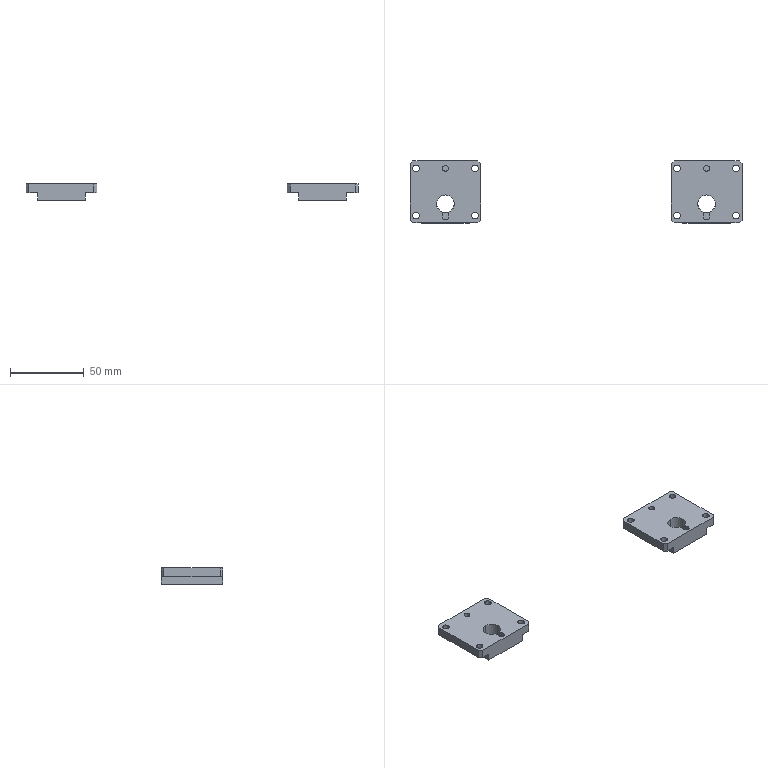NC program | NX | posted with a generic post | part box 225 x 42 x 11 mm
Whole program:
N10 G17 G21 G94 G90
(FLOOR_WALL , TOOL : D63)
N12 T01 M6
N14 G54
N16 G17 G0 G90 X-60.5 Y0. S6500 M3
N18 G43 Z30. H1
N20 Z3.
N22 G94 G1 Z0. F1500.
N24 X-57.5
N26 X57.5
N28 X60.5
N30 Z3.
N32 G0 Z30.
N34 M5
(DRILLING , TOOL : D6A45)
N36 T07 M6
N38 G54
N40 G17 G0 G90 X20. Y-16. S5000 M3
N42 G43 Z30. H7
N44 G94 G81 G98 Z-1. F250. R3.
N46 Y16.
N48 X0.
N50 X-20.
N52 Y-16.
N54 G80
N56 G0 X-20. Y-16. Z30.
N58 M5
(DRILLING_COPY , TOOL : 4.5ZT)
N60 T14 M6
N62 G54
N64 G17 G0 G90 X20. Y-16. S2000 M3
N66 G43 Z30. H14
N68 G94 G83 G98 Z-8.852 F250. Q2. R3.
N70 Y16.
N72 X-20.
N74 Y-16.
N76 G80
N78 G0 X-20. Y-16. Z30.
N80 M5
(ZLEVEL_PROFILE , TOOL : D10)
N82 T10 M6
N84 G54
N86 G17 G0 G90 X1.406 Y-26.1 S9500 M3
N88 G43 Z30. H10
N90 Z1.5
N92 G94 G1 X-22. Z0.273 F1000.
N94 X-22.554 Z0.244
N96 X-23.963 Y-25.74 Z0.168
N98 X-25.215 Y-24.998 Z0.092
N100 X-27.998 Y-22.215 Z-0.114
N102 X-28.74 Y-20.963 Z-0.191
N104 X-29.1 Y-19.554 Z-0.267
N106 Y-19. Z-0.296
N108 Y19. F3000.
N110 G2 X-27.606 Y22.606 R5.1
N112 G1 X-25.606 Y24.606
N114 G2 X-22. Y26.1 R5.1
N116 G1 X22.
N118 G2 X25.606 Y24.606 R5.1
N120 G1 X27.606 Y22.606
N122 G2 X29.1 Y19. R5.1
N124 G1 Y-19.
N126 G2 X27.606 Y-22.606 R5.1
N128 G1 X25.606 Y-24.606
N130 G2 X22. Y-26.1 R5.1
N132 G1 X-22.
N134 G2 X-25.606 Y-24.606 R5.1
N136 G1 X-27.606 Y-22.606
N138 G2 X-29.1 Y-19. R5.1
N140 G1 Y-2.045 Z-0.592
N142 Y19.
N144 G2 X-27.606 Y22.606 R5.1
N146 G1 X-25.606 Y24.606
N148 G2 X-22. Y26.1 R5.1
N150 G1 X22.
N152 G2 X25.606 Y24.606 R5.1
N154 G1 X27.606 Y22.606
N156 G2 X29.1 Y19. R5.1
N158 G1 Y-19.
N160 G2 X27.606 Y-22.606 R5.1
N162 G1 X25.606 Y-24.606
N164 G2 X22. Y-26.1 R5.1
N166 G1 X-22.
N168 G2 X-25.606 Y-24.606 R5.1
N170 G1 X-27.606 Y-22.606
N172 G2 X-29.1 Y-19. R5.1
N174 G1 Y-2.045 Z-0.888
N176 Y19.
N178 G2 X-27.606 Y22.606 R5.1
N180 G1 X-25.606 Y24.606
N182 G2 X-22. Y26.1 R5.1
N184 G1 X22.
N186 G2 X25.606 Y24.606 R5.1
N188 G1 X27.606 Y22.606
N190 G2 X29.1 Y19. R5.1
N192 G1 Y-19.
N194 G2 X27.606 Y-22.606 R5.1
N196 G1 X25.606 Y-24.606
N198 G2 X22. Y-26.1 R5.1
N200 G1 X-22.
N202 G2 X-25.606 Y-24.606 R5.1
N204 G1 X-27.606 Y-22.606
N206 G2 X-29.1 Y-19. R5.1
N208 G1 Y-2.045 Z-1.184
N210 Y19.
N212 G2 X-27.606 Y22.606 R5.1
N214 G1 X-25.606 Y24.606
N216 G2 X-22. Y26.1 R5.1
N218 G1 X22.
N220 G2 X25.606 Y24.606 R5.1
N222 G1 X27.606 Y22.606
N224 G2 X29.1 Y19. R5.1
N226 G1 Y-19.
N228 G2 X27.606 Y-22.606 R5.1
N230 G1 X25.606 Y-24.606
N232 G2 X22. Y-26.1 R5.1
N234 G1 X-22.
N236 G2 X-25.606 Y-24.606 R5.1
N238 G1 X-27.606 Y-22.606
N240 G2 X-29.1 Y-19. R5.1
N242 G1 Y-2.045 Z-1.48
N244 Y19.
N246 G2 X-27.606 Y22.606 R5.1
N248 G1 X-25.606 Y24.606
N250 G2 X-22. Y26.1 R5.1
N252 G1 X22.
N254 G2 X25.606 Y24.606 R5.1
N256 G1 X27.606 Y22.606
N258 G2 X29.1 Y19. R5.1
N260 G1 Y-19.
N262 G2 X27.606 Y-22.606 R5.1
N264 G1 X25.606 Y-24.606
N266 G2 X22. Y-26.1 R5.1
N268 G1 X-22.
N270 G2 X-25.606 Y-24.606 R5.1
N272 G1 X-27.606 Y-22.606
N274 G2 X-29.1 Y-19. R5.1
N276 G1 Y-2.045 Z-1.776
N278 Y19.
N280 G2 X-27.606 Y22.606 R5.1
N282 G1 X-25.606 Y24.606
N284 G2 X-22. Y26.1 R5.1
N286 G1 X22.
N288 G2 X25.606 Y24.606 R5.1
N290 G1 X27.606 Y22.606
N292 G2 X29.1 Y19. R5.1
N294 G1 Y-19.
N296 G2 X27.606 Y-22.606 R5.1
N298 G1 X25.606 Y-24.606
N300 G2 X22. Y-26.1 R5.1
N302 G1 X-22.
N304 G2 X-25.606 Y-24.606 R5.1
N306 G1 X-27.606 Y-22.606
N308 G2 X-29.1 Y-19. R5.1
N310 G1 Y-2.045 Z-2.072
N312 Y19.
N314 G2 X-27.606 Y22.606 R5.1
N316 G1 X-25.606 Y24.606
N318 G2 X-22. Y26.1 R5.1
N320 G1 X22.
N322 G2 X25.606 Y24.606 R5.1
N324 G1 X27.606 Y22.606
N326 G2 X29.1 Y19. R5.1
N328 G1 Y-19.
N330 G2 X27.606 Y-22.606 R5.1
N332 G1 X25.606 Y-24.606
N334 G2 X22. Y-26.1 R5.1
N336 G1 X-22.
N338 G2 X-25.606 Y-24.606 R5.1
N340 G1 X-27.606 Y-22.606
N342 G2 X-29.1 Y-19. R5.1
N344 G1 Y-2.045 Z-2.368
N346 Y19.
N348 G2 X-27.606 Y22.606 R5.1
N350 G1 X-25.606 Y24.606
N352 G2 X-22. Y26.1 R5.1
N354 G1 X22.
N356 G2 X25.606 Y24.606 R5.1
N358 G1 X27.606 Y22.606
N360 G2 X29.1 Y19. R5.1
N362 G1 Y-19.
N364 G2 X27.606 Y-22.606 R5.1
N366 G1 X25.606 Y-24.606
N368 G2 X22. Y-26.1 R5.1
N370 G1 X-22.
N372 G2 X-25.606 Y-24.606 R5.1
N374 G1 X-27.606 Y-22.606
N376 G2 X-29.1 Y-19. R5.1
N378 G1 Y-2.045 Z-2.664
N380 Y19.
N382 G2 X-27.606 Y22.606 R5.1
N384 G1 X-25.606 Y24.606
N386 G2 X-22. Y26.1 R5.1
N388 G1 X22.
N390 G2 X25.606 Y24.606 R5.1
N392 G1 X27.606 Y22.606
N394 G2 X29.1 Y19. R5.1
N396 G1 Y-19.
N398 G2 X27.606 Y-22.606 R5.1
N400 G1 X25.606 Y-24.606
N402 G2 X22. Y-26.1 R5.1
N404 G1 X-22.
N406 G2 X-25.606 Y-24.606 R5.1
N408 G1 X-27.606 Y-22.606
N410 G2 X-29.1 Y-19. R5.1
N412 G1 Y-2.045 Z-2.959
N414 Y19.
N416 G2 X-27.606 Y22.606 R5.1
N418 G1 X-25.606 Y24.606
N420 G2 X-22. Y26.1 R5.1
N422 G1 X22.
N424 G2 X25.606 Y24.606 R5.1
N426 G1 X27.606 Y22.606
N428 G2 X29.1 Y19. R5.1
N430 G1 Y-19.
N432 G2 X27.606 Y-22.606 R5.1
N434 G1 X25.606 Y-24.606
N436 G2 X22. Y-26.1 R5.1
N438 G1 X-22.
N440 G2 X-25.606 Y-24.606 R5.1
N442 G1 X-27.606 Y-22.606
N444 G2 X-29.1 Y-19. R5.1
N446 G1 Y-2.045 Z-3.255
N448 Y19.
N450 G2 X-27.606 Y22.606 R5.1
N452 G1 X-25.606 Y24.606
N454 G2 X-22. Y26.1 R5.1
N456 G1 X22.
N458 G2 X25.606 Y24.606 R5.1
N460 G1 X27.606 Y22.606
N462 G2 X29.1 Y19. R5.1
N464 G1 Y-19.
N466 G2 X27.606 Y-22.606 R5.1
N468 G1 X25.606 Y-24.606
N470 G2 X22. Y-26.1 R5.1
N472 G1 X-22.
N474 G2 X-25.606 Y-24.606 R5.1
N476 G1 X-27.606 Y-22.606
N478 G2 X-29.1 Y-19. R5.1
N480 G1 Y-2.045 Z-3.551
N482 Y19.
N484 G2 X-27.606 Y22.606 R5.1
N486 G1 X-25.606 Y24.606
N488 G2 X-22. Y26.1 R5.1
N490 G1 X22.
N492 G2 X25.606 Y24.606 R5.1
N494 G1 X27.606 Y22.606
N496 G2 X29.1 Y19. R5.1
N498 G1 Y-19.
N500 G2 X27.606 Y-22.606 R5.1
N502 G1 X25.606 Y-24.606
N504 G2 X22. Y-26.1 R5.1
N506 G1 X-22.
N508 G2 X-25.606 Y-24.606 R5.1
N510 G1 X-27.606 Y-22.606
N512 G2 X-29.1 Y-19. R5.1
N514 G1 Y-2.045 Z-3.847
N516 Y19.
N518 G2 X-27.606 Y22.606 R5.1
N520 G1 X-25.606 Y24.606
N522 G2 X-22. Y26.1 R5.1
N524 G1 X22.
N526 G2 X25.606 Y24.606 R5.1
N528 G1 X27.606 Y22.606
N530 G2 X29.1 Y19. R5.1
N532 G1 Y-19.
N534 G2 X27.606 Y-22.606 R5.1
N536 G1 X25.606 Y-24.606
N538 G2 X22. Y-26.1 R5.1
N540 G1 X-22.
N542 G2 X-25.606 Y-24.606 R5.1
N544 G1 X-27.606 Y-22.606
N546 G2 X-29.1 Y-19. R5.1
N548 G1 Y-2.045 Z-4.143
N550 Y19.
N552 G2 X-27.606 Y22.606 R5.1
N554 G1 X-25.606 Y24.606
N556 G2 X-22. Y26.1 R5.1
N558 G1 X22.
N560 G2 X25.606 Y24.606 R5.1
N562 G1 X27.606 Y22.606
N564 G2 X29.1 Y19. R5.1
N566 G1 Y-19.
N568 G2 X27.606 Y-22.606 R5.1
N570 G1 X25.606 Y-24.606
N572 G2 X22. Y-26.1 R5.1
N574 G1 X-22.
N576 G2 X-25.606 Y-24.606 R5.1
N578 G1 X-27.606 Y-22.606
N580 G2 X-29.1 Y-19. R5.1
N582 G1 Y-2.045 Z-4.439
N584 Y19.
N586 G2 X-27.606 Y22.606 R5.1
N588 G1 X-25.606 Y24.606
N590 G2 X-22. Y26.1 R5.1
N592 G1 X22.
N594 G2 X25.606 Y24.606 R5.1
N596 G1 X27.606 Y22.606
N598 G2 X29.1 Y19. R5.1
N600 G1 Y-19.
N602 G2 X27.606 Y-22.606 R5.1
N604 G1 X25.606 Y-24.606
N606 G2 X22. Y-26.1 R5.1
N608 G1 X-22.
N610 G2 X-25.606 Y-24.606 R5.1
N612 G1 X-27.606 Y-22.606
N614 G2 X-29.1 Y-19. R5.1
N616 G1 Y-2.045 Z-4.735
N618 Y19.
N620 G2 X-27.606 Y22.606 R5.1
N622 G1 X-25.606 Y24.606
N624 G2 X-22. Y26.1 R5.1
N626 G1 X22.
N628 G2 X25.606 Y24.606 R5.1
N630 G1 X27.606 Y22.606
N632 G2 X29.1 Y19. R5.1
N634 G1 Y-19.
N636 G2 X27.606 Y-22.606 R5.1
N638 G1 X25.606 Y-24.606
N640 G2 X22. Y-26.1 R5.1
N642 G1 X-22.
N644 G2 X-25.606 Y-24.606 R5.1
N646 G1 X-27.606 Y-22.606
N648 G2 X-29.1 Y-19. R5.1
N650 G1 Y-2.045 Z-5.031
N652 Y19.
N654 G2 X-27.606 Y22.606 R5.1
N656 G1 X-25.606 Y24.606
N658 G2 X-22. Y26.1 R5.1
N660 G1 X22.
N662 G2 X25.606 Y24.606 R5.1
N664 G1 X27.606 Y22.606
N666 G2 X29.1 Y19. R5.1
N668 G1 Y-19.
N670 G2 X27.606 Y-22.606 R5.1
N672 G1 X25.606 Y-24.606
N674 G2 X22. Y-26.1 R5.1
N676 G1 X-22.
N678 G2 X-25.606 Y-24.606 R5.1
N680 G1 X-27.606 Y-22.606
N682 G2 X-29.1 Y-19. R5.1
N684 G1 Y-2.045 Z-5.327
N686 Y19.
N688 G2 X-27.606 Y22.606 R5.1
N690 G1 X-25.606 Y24.606
N692 G2 X-22. Y26.1 R5.1
N694 G1 X22.
N696 G2 X25.606 Y24.606 R5.1
N698 G1 X27.606 Y22.606
N700 G2 X29.1 Y19. R5.1
N702 G1 Y-19.
N704 G2 X27.606 Y-22.606 R5.1
N706 G1 X25.606 Y-24.606
N708 G2 X22. Y-26.1 R5.1
N710 G1 X-22.
N712 G2 X-25.606 Y-24.606 R5.1
N714 G1 X-27.606 Y-22.606
N716 G2 X-29.1 Y-19. R5.1
N718 G1 Y-2.045 Z-5.623
N720 Y19.
N722 G2 X-27.606 Y22.606 R5.1
N724 G1 X-25.606 Y24.606
N726 G2 X-22. Y26.1 R5.1
N728 G1 X22.
N730 G2 X25.606 Y24.606 R5.1
N732 G1 X27.606 Y22.606
N734 G2 X29.1 Y19. R5.1
N736 G1 Y-19.
N738 G2 X27.606 Y-22.606 R5.1
N740 G1 X25.606 Y-24.606
N742 G2 X22. Y-26.1 R5.1
N744 G1 X-22.
N746 G2 X-25.606 Y-24.606 R5.1
N748 G1 X-27.606 Y-22.606
N750 G2 X-29.1 Y-19. R5.1
N752 G1 Y-2.045 Z-5.919
N754 Y19.
N756 G2 X-27.606 Y22.606 R5.1
N758 G1 X-25.606 Y24.606
N760 G2 X-22. Y26.1 R5.1
N762 G1 X22.
N764 G2 X25.606 Y24.606 R5.1
N766 G1 X27.606 Y22.606
N768 G2 X29.1 Y19. R5.1
N770 G1 Y-19.
N772 G2 X27.606 Y-22.606 R5.1
N774 G1 X25.606 Y-24.606
N776 G2 X22. Y-26.1 R5.1
N778 G1 X-22.
N780 G2 X-25.606 Y-24.606 R5.1
N782 G1 X-27.606 Y-22.606
N784 G2 X-29.1 Y-19. R5.1
N786 G1 Y-2.045 Z-6.215
N788 Y19.
N790 G2 X-27.606 Y22.606 R5.1
N792 G1 X-25.606 Y24.606
N794 G2 X-22. Y26.1 R5.1
N796 G1 X22.
N798 G2 X25.606 Y24.606 R5.1
N800 G1 X27.606 Y22.606
N802 G2 X29.1 Y19. R5.1
N804 G1 Y-19.
N806 G2 X27.606 Y-22.606 R5.1
N808 G1 X25.606 Y-24.606
N810 G2 X22. Y-26.1 R5.1
N812 G1 X-22.
N814 G2 X-25.606 Y-24.606 R5.1
N816 G1 X-27.606 Y-22.606
N818 G2 X-29.1 Y-19. R5.1
N820 G1 Y-2.045 Z-6.511
N822 Y19.
N824 G2 X-27.606 Y22.606 R5.1
N826 G1 X-25.606 Y24.606
N828 G2 X-22. Y26.1 R5.1
N830 G1 X22.
N832 G2 X25.606 Y24.606 R5.1
N834 G1 X27.606 Y22.606
N836 G2 X29.1 Y19. R5.1
N838 G1 Y-19.
N840 G2 X27.606 Y-22.606 R5.1
N842 G1 X25.606 Y-24.606
N844 G2 X22. Y-26.1 R5.1
N846 G1 X-22.
N848 G2 X-25.606 Y-24.606 R5.1
N850 G1 X-27.606 Y-22.606
N852 G2 X-29.1 Y-19. R5.1
N854 G1 Y-2.045 Z-6.807
N856 Y19.
N858 G2 X-27.606 Y22.606 R5.1
N860 G1 X-25.606 Y24.606
N862 G2 X-22. Y26.1 R5.1
N864 G1 X22.
N866 G2 X25.606 Y24.606 R5.1
N868 G1 X27.606 Y22.606
N870 G2 X29.1 Y19. R5.1
N872 G1 Y-19.
N874 G2 X27.606 Y-22.606 R5.1
N876 G1 X25.606 Y-24.606
N878 G2 X22. Y-26.1 R5.1
N880 G1 X-22.
N882 G2 X-25.606 Y-24.606 R5.1
N884 G1 X-27.606 Y-22.606
N886 G2 X-29.1 Y-19. R5.1
N888 G1 Y-2.045 Z-7.103
N890 Y19.
N892 G2 X-27.606 Y22.606 R5.1
N894 G1 X-25.606 Y24.606
N896 G2 X-22. Y26.1 R5.1
N898 G1 X22.
N900 G2 X25.606 Y24.606 R5.1
N902 G1 X27.606 Y22.606
N904 G2 X29.1 Y19. R5.1
N906 G1 Y-19.
N908 G2 X27.606 Y-22.606 R5.1
N910 G1 X25.606 Y-24.606
N912 G2 X22. Y-26.1 R5.1
N914 G1 X-22.
N916 G2 X-25.606 Y-24.606 R5.1
N918 G1 X-27.606 Y-22.606
N920 G2 X-29.1 Y-19. R5.1
N922 G1 Y-2.045 Z-7.399
N924 Y19.
N926 G2 X-27.606 Y22.606 R5.1
N928 G1 X-25.606 Y24.606
N930 G2 X-22. Y26.1 R5.1
N932 G1 X22.
N934 G2 X25.606 Y24.606 R5.1
N936 G1 X27.606 Y22.606
N938 G2 X29.1 Y19. R5.1
N940 G1 Y-19.
N942 G2 X27.606 Y-22.606 R5.1
N944 G1 X25.606 Y-24.606
N946 G2 X22. Y-26.1 R5.1
N948 G1 X-22.
N950 G2 X-25.606 Y-24.606 R5.1
N952 G1 X-27.606 Y-22.606
N954 G2 X-29.1 Y-19. R5.1
N956 G1 Y-2.045 Z-7.695
N958 Y19.
N960 G2 X-27.606 Y22.606 R5.1
N962 G1 X-25.606 Y24.606
N964 G2 X-22. Y26.1 R5.1
N966 G1 X22.
N968 G2 X25.606 Y24.606 R5.1
N970 G1 X27.606 Y22.606
N972 G2 X29.1 Y19. R5.1
N974 G1 Y-19.
N976 G2 X27.606 Y-22.606 R5.1
N978 G1 X25.606 Y-24.606
N980 G2 X22. Y-26.1 R5.1
N982 G1 X-22.
N984 G2 X-25.606 Y-24.606 R5.1
N986 G1 X-27.606 Y-22.606
N988 G2 X-29.1 Y-19. R5.1
N990 G1 Y-2.045 Z-7.991
N992 Y19.
N994 G2 X-27.606 Y22.606 R5.1
N996 G1 X-25.606 Y24.606
N998 G2 X-22. Y26.1 R5.1
N1000 G1 X22.
N1002 G2 X25.606 Y24.606 R5.1
N1004 G1 X27.606 Y22.606
N1006 G2 X29.1 Y19. R5.1
N1008 G1 Y-19.
N1010 G2 X27.606 Y-22.606 R5.1
N1012 G1 X25.606 Y-24.606
N1014 G2 X22. Y-26.1 R5.1
N1016 G1 X-22.
N1018 G2 X-25.606 Y-24.606 R5.1
N1020 G1 X-27.606 Y-22.606
N1022 G2 X-29.1 Y-19. R5.1
N1024 G1 Y-2.045 Z-8.286
N1026 Y19.
N1028 G2 X-27.606 Y22.606 R5.1
N1030 G1 X-25.606 Y24.606
N1032 G2 X-22. Y26.1 R5.1
N1034 G1 X22.
N1036 G2 X25.606 Y24.606 R5.1
N1038 G1 X27.606 Y22.606
N1040 G2 X29.1 Y19. R5.1
N1042 G1 Y-19.
N1044 G2 X27.606 Y-22.606 R5.1
N1046 G1 X25.606 Y-24.606
N1048 G2 X22. Y-26.1 R5.1
N1050 G1 X-22.
N1052 G2 X-25.606 Y-24.606 R5.1
N1054 G1 X-27.606 Y-22.606
N1056 G2 X-29.1 Y-19. R5.1
N1058 G1 Y-2.045 Z-8.582
N1060 Y19.
N1062 G2 X-27.606 Y22.606 R5.1
N1064 G1 X-25.606 Y24.606
N1066 G2 X-22. Y26.1 R5.1
N1068 G1 X22.
N1070 G2 X25.606 Y24.606 R5.1
N1072 G1 X27.606 Y22.606
N1074 G2 X29.1 Y19. R5.1
N1076 G1 Y-19.
N1078 G2 X27.606 Y-22.606 R5.1
N1080 G1 X25.606 Y-24.606
N1082 G2 X22. Y-26.1 R5.1
N1084 G1 X-22.
N1086 G2 X-25.606 Y-24.606 R5.1
N1088 G1 X-27.606 Y-22.606
N1090 G2 X-29.1 Y-19. R5.1
N1092 G1 Y-2.045 Z-8.878
N1094 Y19.
N1096 G2 X-27.606 Y22.606 R5.1
N1098 G1 X-25.606 Y24.606
N1100 G2 X-22. Y26.1 R5.1
N1102 G1 X22.
N1104 G2 X25.606 Y24.606 R5.1
N1106 G1 X27.606 Y22.606
N1108 G2 X29.1 Y19. R5.1
N1110 G1 Y-19.
N1112 G2 X27.606 Y-22.606 R5.1
N1114 G1 X25.606 Y-24.606
N1116 G2 X22. Y-26.1 R5.1
N1118 G1 X-22.
N1120 G2 X-25.606 Y-24.606 R5.1
N1122 G1 X-27.606 Y-22.606
N1124 G2 X-29.1 Y-19. R5.1
N1126 G1 Y-2.045 Z-9.174
N1128 Y19.
N1130 G2 X-27.606 Y22.606 R5.1
N1132 G1 X-25.606 Y24.606
N1134 G2 X-22. Y26.1 R5.1
N1136 G1 X22.
N1138 G2 X25.606 Y24.606 R5.1
N1140 G1 X27.606 Y22.606
N1142 G2 X29.1 Y19. R5.1
N1144 G1 Y-19.
N1146 G2 X27.606 Y-22.606 R5.1
N1148 G1 X25.606 Y-24.606
N1150 G2 X22. Y-26.1 R5.1
N1152 G1 X-22.
N1154 G2 X-25.606 Y-24.606 R5.1
N1156 G1 X-27.606 Y-22.606
N1158 G2 X-29.1 Y-19. R5.1
N1160 G1 Y-2.045 Z-9.47
N1162 Y19.
N1164 G2 X-27.606 Y22.606 R5.1
N1166 G1 X-25.606 Y24.606
N1168 G2 X-22. Y26.1 R5.1
N1170 G1 X22.
N1172 G2 X25.606 Y24.606 R5.1
N1174 G1 X27.606 Y22.606
N1176 G2 X29.1 Y19. R5.1
N1178 G1 Y-19.
N1180 G2 X27.606 Y-22.606 R5.1
N1182 G1 X25.606 Y-24.606
N1184 G2 X22. Y-26.1 R5.1
N1186 G1 X-22.
N1188 G2 X-25.606 Y-24.606 R5.1
N1190 G1 X-27.606 Y-22.606
N1192 G2 X-29.1 Y-19. R5.1
N1194 G1 Y-2.045 Z-9.766
N1196 Y19.
N1198 G2 X-27.606 Y22.606 R5.1
N1200 G1 X-25.606 Y24.606
N1202 G2 X-22. Y26.1 R5.1
N1204 G1 X22.
N1206 G2 X25.606 Y24.606 R5.1
N1208 G1 X27.606 Y22.606
N1210 G2 X29.1 Y19. R5.1
N1212 G1 Y-19.
N1214 G2 X27.606 Y-22.606 R5.1
N1216 G1 X25.606 Y-24.606
N1218 G2 X22. Y-26.1 R5.1
N1220 G1 X-22.
N1222 G2 X-25.606 Y-24.606 R5.1
N1224 G1 X-27.606 Y-22.606
N1226 G2 X-29.1 Y-19. R5.1
N1228 G1 Y-2.045 Z-10.062
N1230 Y19.
N1232 G2 X-27.606 Y22.606 R5.1
N1234 G1 X-25.606 Y24.606
N1236 G2 X-22. Y26.1 R5.1
N1238 G1 X22.
N1240 G2 X25.606 Y24.606 R5.1
N1242 G1 X27.606 Y22.606
N1244 G2 X29.1 Y19. R5.1
N1246 G1 Y-19.
N1248 G2 X27.606 Y-22.606 R5.1
N1250 G1 X25.606 Y-24.606
N1252 G2 X22. Y-26.1 R5.1
N1254 G1 X-22.
N1256 G2 X-25.606 Y-24.606 R5.1
N1258 G1 X-27.606 Y-22.606
N1260 G2 X-29.1 Y-19. R5.1
N1262 G1 Y-2.045 Z-10.358
N1264 Y19.
N1266 G2 X-27.606 Y22.606 R5.1
N1268 G1 X-25.606 Y24.606
N1270 G2 X-22. Y26.1 R5.1
N1272 G1 X22.
N1274 G2 X25.606 Y24.606 R5.1
N1276 G1 X27.606 Y22.606
N1278 G2 X29.1 Y19. R5.1
N1280 G1 Y-19.
N1282 G2 X27.606 Y-22.606 R5.1
N1284 G1 X25.606 Y-24.606
N1286 G2 X22. Y-26.1 R5.1
N1288 G1 X-22.
N1290 G2 X-25.606 Y-24.606 R5.1
N1292 G1 X-27.606 Y-22.606
N1294 G2 X-29.1 Y-19. R5.1
N1296 G1 Y-2.045 Z-10.654
N1298 Y19.
N1300 G2 X-27.606 Y22.606 R5.1
N1302 G1 X-25.606 Y24.606
N1304 G2 X-22. Y26.1 R5.1
N1306 G1 X22.
N1308 G2 X25.606 Y24.606 R5.1
N1310 G1 X27.606 Y22.606
N1312 G2 X29.1 Y19. R5.1
N1314 G1 Y-19.
N1316 G2 X27.606 Y-22.606 R5.1
N1318 G1 X25.606 Y-24.606
N1320 G2 X22. Y-26.1 R5.1
N1322 G1 X-22.
N1324 G2 X-25.606 Y-24.606 R5.1
N1326 G1 X-27.606 Y-22.606
N1328 G2 X-29.1 Y-19. R5.1
N1330 G1 Y-2.045 Z-10.95
N1332 Y19.
N1334 G2 X-27.606 Y22.606 R5.1
N1336 G1 X-25.606 Y24.606
N1338 G2 X-22. Y26.1 R5.1
N1340 G1 X22.
N1342 G2 X25.606 Y24.606 R5.1
N1344 G1 X27.606 Y22.606
N1346 G2 X29.1 Y19. R5.1
N1348 G1 Y-19.
N1350 G2 X27.606 Y-22.606 R5.1
N1352 G1 X25.606 Y-24.606
N1354 G2 X22. Y-26.1 R5.1
N1356 G1 X-22.
N1358 G2 X-25.606 Y-24.606 R5.1
N1360 G1 X-27.606 Y-22.606
N1362 G2 X-29.1 Y-19. R5.1
N1364 G1 Y-2.045
N1366 Z-9.45
N1368 G0 Z30.
(HOLE_MILLING , TOOL : D10)
N1370 X0. Y-8.
N1372 Z0.5
N1374 G3 X0.45 Y-8.45 R0.45 F2000.
N1376 X0.9 Y-8. R0.45
N1378 X0.9 Y-8. Z0.2 I-0.9 J0.
N1380 X0.9 Y-8. Z-0.1 I-0.9 J0.
N1382 X0.9 Y-8. Z-0.4 I-0.9 J0.
N1384 X0.9 Y-8. Z-0.7 I-0.9 J0.
N1386 X0.9 Y-8. Z-1. I-0.9 J0.
N1388 X0.9 Y-8. Z-1.3 I-0.9 J0.
N1390 X0.9 Y-8. Z-1.6 I-0.9 J0.
N1392 X0.9 Y-8. Z-1.9 I-0.9 J0.
N1394 X0.9 Y-8. Z-2.2 I-0.9 J0.
N1396 X0.9 Y-8. Z-2.5 I-0.9 J0.
N1398 X0.9 Y-8. Z-2.8 I-0.9 J0.
N1400 X0.9 Y-8. Z-3.1 I-0.9 J0.
N1402 X0.9 Y-8. Z-3.4 I-0.9 J0.
N1404 X0.9 Y-8. Z-3.7 I-0.9 J0.
N1406 X0.9 Y-8. Z-4. I-0.9 J0.
N1408 X0.9 Y-8. Z-4.3 I-0.9 J0.
N1410 X0.9 Y-8. Z-4.6 I-0.9 J0.
N1412 X0.9 Y-8. Z-4.9 I-0.9 J0.
N1414 X0.9 Y-8. Z-5.2 I-0.9 J0.
N1416 X0.9 Y-8. Z-5.5 I-0.9 J0.
N1418 X0.9 Y-8. Z-5.8 I-0.9 J0.
N1420 X0.9 Y-8. Z-6.1 I-0.9 J0.
N1422 X0.9 Y-8. Z-6.4 I-0.9 J0.
N1424 X0.9 Y-8. Z-6.7 I-0.9 J0.
N1426 X0.9 Y-8. Z-7. I-0.9 J0.
N1428 X0.9 Y-8. Z-7.3 I-0.9 J0.
N1430 X0.9 Y-8. Z-7.6 I-0.9 J0.
N1432 X0.9 Y-8. Z-7.9 I-0.9 J0.
N1434 X0.9 Y-8. Z-8.2 I-0.9 J0.
N1436 X0.9 Y-8. Z-8.5 I-0.9 J0.
N1438 X0.9 Y-8. Z-8.8 I-0.9 J0.
N1440 X0.9 Y-8. Z-9.1 I-0.9 J0.
N1442 X0.9 Y-8. Z-9.4 I-0.9 J0.
N1444 X0.9 Y-8. Z-9.7 I-0.9 J0.
N1446 X0.9 Y-8. Z-10. I-0.9 J0.
N1448 X0.9 Y-8. Z-10.3 I-0.9 J0.
N1450 X0.9 Y-8. Z-10.6 I-0.9 J0.
N1452 X0.9 Y-8. Z-10.9 I-0.9 J0.
N1454 X-0.45 Y-7.221 Z-11. R0.9
N1456 X-0.779 Y-8.45 R0.9
N1458 X-0.45 Y-7.221 R-0.9
N1460 X-0.615 Y-7.835 R0.45
N1462 X0. Y-8. R0.45
N1464 G0 Z30.
N1466 M5
(HOLE_MILLING_COPY , TOOL : D10JING)
N1468 T11 M6
N1470 G54
N1472 G17 G0 G90 X0. Y-8. S9500 M3
N1474 G43 Z30. H11
N1476 Z0.5
N1478 G94 G3 X0.5 Y-8.5 R0.5 F1200.
N1480 X1. Y-8. R0.5
N1482 X1. Y-8. Z-4.5 I-1. J0.
N1484 X1. Y-8. Z-9.5 I-1. J0.
N1486 X-0.309 Y-7.049 Z-11. R1.
N1488 X-0.951 Y-8.309 R1.
N1490 X-0.309 Y-7.049 R-1.
N1492 X-0.63 Y-7.679 R0.5
N1494 X0. Y-8. R0.5
N1496 G0 Z30.
N1498 M5
(HOLE_MILLING_1 , TOOL : D3)
N1500 T03 M6
N1502 G54
N1504 G17 G0 G90 X0. Y16. S9500 M3
N1506 G43 Z30. H3
N1508 Z0.5
N1510 G94 G3 X0.2 Y15.8 R0.2 F1250.
N1512 X0.4 Y16. R0.2
N1514 X0.4 Y16. Z0.35 I-0.4 J0.
N1516 X0.4 Y16. Z0.2 I-0.4 J0.
N1518 X0.4 Y16. Z0.05 I-0.4 J0.
N1520 X0.4 Y16. Z-0.1 I-0.4 J0.
N1522 X0.4 Y16. Z-0.25 I-0.4 J0.
N1524 X0.4 Y16. Z-0.4 I-0.4 J0.
N1526 X0.4 Y16. Z-0.55 I-0.4 J0.
N1528 X0.4 Y16. Z-0.7 I-0.4 J0.
N1530 X0.4 Y16. Z-0.85 I-0.4 J0.
N1532 X0.4 Y16. Z-1. I-0.4 J0.
N1534 X0.4 Y16. Z-1.15 I-0.4 J0.
N1536 X0.4 Y16. Z-1.3 I-0.4 J0.
N1538 X0.4 Y16. Z-1.45 I-0.4 J0.
N1540 X0.4 Y16. Z-1.6 I-0.4 J0.
N1542 X0.4 Y16. Z-1.75 I-0.4 J0.
N1544 X0.4 Y16. Z-1.9 I-0.4 J0.
N1546 X0.4 Y16. Z-2.05 I-0.4 J0.
N1548 X0.4 Y16. Z-2.2 I-0.4 J0.
N1550 X0.4 Y16. Z-2.35 I-0.4 J0.
N1552 X0.4 Y16. Z-2.5 I-0.4 J0.
N1554 X0.4 Y16. Z-2.65 I-0.4 J0.
N1556 X0.4 Y16. Z-2.8 I-0.4 J0.
N1558 X0.4 Y16. Z-2.95 I-0.4 J0.
N1560 X0.4 Y16. Z-3.1 I-0.4 J0.
N1562 X0.4 Y16. Z-3.25 I-0.4 J0.
N1564 X0.4 Y16. Z-3.4 I-0.4 J0.
N1566 X0.4 Y16. Z-3.55 I-0.4 J0.
N1568 X0.4 Y16. Z-3.7 I-0.4 J0.
N1570 X0.4 Y16. Z-3.85 I-0.4 J0.
N1572 X0.4 Y16. Z-4. I-0.4 J0.
N1574 X0.4 Y16. Z-4.15 I-0.4 J0.
N1576 X0.4 Y16. Z-4.3 I-0.4 J0.
N1578 X0.4 Y16. Z-4.45 I-0.4 J0.
N1580 X0.4 Y16. Z-4.6 I-0.4 J0.
N1582 X0.4 Y16. Z-4.75 I-0.4 J0.
N1584 X0.4 Y16. Z-4.9 I-0.4 J0.
N1586 X0.4 Y16. Z-5.05 I-0.4 J0.
N1588 X0.4 Y16. Z-5.2 I-0.4 J0.
N1590 X0.4 Y16. Z-5.35 I-0.4 J0.
N1592 X0.4 Y16. Z-5.5 I-0.4 J0.
N1594 X0.4 Y16. Z-5.65 I-0.4 J0.
N1596 X0.4 Y16. Z-5.8 I-0.4 J0.
N1598 X0.4 Y16. Z-5.95 I-0.4 J0.
N1600 X-0.2 Y16.346 Z-6. R0.4
N1602 X-0.346 Y15.8 R0.4
N1604 X-0.2 Y16.346 R-0.4
N1606 X-0.273 Y16.073 R0.2
N1608 X0. Y16. R0.2
N1610 G0 Z30.
(ZLEVEL_PROFILE_1 , TOOL : D3)
N1612 Y-11.097
N1614 Z-0.15
N1616 G1 X-0.256 Y-11.895 F1500.
N1618 G3 X-0.403 Y-12.157 R0.3
N1620 G1 X-0.4 Y-12.41
N1622 Y-13.667
N1624 Y-17.
N1626 G3 X0. Y-17.4 R0.4
N1628 X0.4 Y-17. R0.4
N1630 G1 Y-13.657
N1632 X0.419 Y-13.408
N1634 X0.4 Y-13.389
N1636 X0.403 Y-12.157
N1638 G3 X0.254 Y-11.897 R0.3
N1640 G1 X0. Y-11.097
N1642 G0 Z-0.3
N1644 G1 X-0.255 Y-11.895
N1646 G3 X-0.403 Y-12.157 R0.3
N1648 G1 X-0.4 Y-12.41
N1650 Y-13.667
N1652 Y-17.
N1654 G3 X0. Y-17.4 R0.4
N1656 X0.4 Y-17. R0.4
N1658 G1 Y-13.657
N1660 X0.419 Y-13.408
N1662 X0.4 Y-13.389
N1664 X0.403 Y-12.157
N1666 G3 X0.254 Y-11.897 R0.3
N1668 G1 X0. Y-11.097
N1670 G0 Y-11.096 Z-0.45
N1672 G1 X-0.255 Y-11.896
N1674 G3 X-0.402 Y-12.157 R0.3
N1676 G1 X-0.4 Y-12.41
N1678 Y-13.667
N1680 Y-17.
N1682 G3 X0. Y-17.4 R0.4
N1684 X0.4 Y-17. R0.4
N1686 G1 Y-13.657
N1688 X0.419 Y-13.408
N1690 X0.4 Y-13.389
N1692 X0.403 Y-12.157
N1694 G3 X0.253 Y-11.897 R0.3
N1696 G1 X0. Y-11.096
N1698 G0 Z-0.6
N1700 G1 X-0.255 Y-11.896
N1702 G3 X-0.402 Y-12.157 R0.3
N1704 G1 X-0.4 Y-12.41
N1706 Y-13.667
N1708 Y-17.
N1710 G3 X0. Y-17.4 R0.4
N1712 X0.4 Y-17. R0.4
N1714 G1 Y-13.657
N1716 X0.419 Y-13.408
N1718 X0.4 Y-13.389
N1720 X0.403 Y-12.157
N1722 G3 X0.253 Y-11.897 R0.3
N1724 G1 X0. Y-11.096
N1726 G0 Z-0.75
N1728 G1 X-0.255 Y-11.896
N1730 G3 X-0.402 Y-12.157 R0.3
N1732 G1 X-0.4 Y-12.41
N1734 Y-13.667
N1736 Y-17.
N1738 G3 X0. Y-17.4 R0.4
N1740 X0.4 Y-17. R0.4
N1742 G1 Y-13.657
N1744 X0.419 Y-13.408
N1746 X0.4 Y-13.389
N1748 X0.403 Y-12.157
N1750 G3 X0.253 Y-11.897 R0.3
N1752 G1 X0. Y-11.096
N1754 G0 Z-0.9
N1756 G1 X-0.255 Y-11.896
N1758 G3 X-0.402 Y-12.157 R0.3
N1760 G1 X-0.4 Y-12.41
N1762 Y-13.667
N1764 Y-17.
N1766 G3 X0. Y-17.4 R0.4
N1768 X0.4 Y-17. R0.4
N1770 G1 Y-13.657
N1772 X0.419 Y-13.408
N1774 X0.4 Y-13.389
N1776 X0.403 Y-12.157
N1778 G3 X0.253 Y-11.897 R0.3
N1780 G1 X0. Y-11.096
N1782 G0 Z-1.05
N1784 G1 X-0.255 Y-11.896
N1786 G3 X-0.402 Y-12.157 R0.3
N1788 G1 X-0.399 Y-12.41
N1790 X-0.4 Y-13.667
N1792 Y-17.
N1794 G3 X0. Y-17.4 R0.4
N1796 X0.4 Y-17. R0.4
N1798 G1 X0.399 Y-13.657
N1800 X0.419 Y-13.408
N1802 X0.399 Y-13.389
N1804 X0.403 Y-12.157
N1806 G3 X0.253 Y-11.897 R0.3
N1808 G1 X0. Y-11.096
N1810 G0 Z-1.2
N1812 G1 X-0.255 Y-11.896
N1814 G3 X-0.402 Y-12.157 R0.3
N1816 G1 X-0.399 Y-12.41
N1818 X-0.4 Y-13.667
N1820 Y-17.
N1822 G3 X0. Y-17.4 R0.4
N1824 X0.4 Y-17. R0.4
N1826 G1 X0.399 Y-13.657
N1828 X0.419 Y-13.408
N1830 X0.399 Y-13.389
N1832 X0.403 Y-12.157
N1834 G3 X0.253 Y-11.897 R0.3
N1836 G1 X0. Y-11.096
N1838 G0 Z-1.35
N1840 G1 X-0.255 Y-11.896
N1842 G3 X-0.402 Y-12.157 R0.3
N1844 G1 X-0.399 Y-12.41
N1846 X-0.4 Y-13.667
N1848 Y-17.
N1850 G3 X0. Y-17.4 R0.4
N1852 X0.4 Y-17. R0.4
N1854 G1 X0.399 Y-13.657
N1856 X0.419 Y-13.408
N1858 X0.399 Y-13.389
N1860 X0.403 Y-12.157
N1862 G3 X0.253 Y-11.897 R0.3
N1864 G1 X0. Y-11.096
N1866 G0 Z-1.5
N1868 G1 X-0.255 Y-11.896
N1870 G3 X-0.402 Y-12.157 R0.3
N1872 G1 X-0.399 Y-12.41
N1874 X-0.4 Y-13.667
N1876 Y-17.
N1878 G3 X0. Y-17.4 R0.4
N1880 X0.4 Y-17. R0.4
N1882 G1 X0.399 Y-13.657
N1884 X0.419 Y-13.408
N1886 X0.399 Y-13.389
N1888 X0.403 Y-12.157
N1890 G3 X0.253 Y-11.897 R0.3
N1892 G1 X0. Y-11.096
N1894 G0 Z-1.65
N1896 G1 X-0.255 Y-11.896
N1898 G3 X-0.402 Y-12.157 R0.3
N1900 G1 X-0.399 Y-12.41
N1902 X-0.4 Y-13.667
N1904 Y-17.
N1906 G3 X0. Y-17.4 R0.4
N1908 X0.4 Y-17. R0.4
N1910 G1 X0.399 Y-13.657
N1912 X0.419 Y-13.408
N1914 X0.399 Y-13.389
N1916 X0.403 Y-12.157
N1918 G3 X0.253 Y-11.897 R0.3
N1920 G1 X0. Y-11.096
N1922 G0 Z-1.8
N1924 G1 X-0.255 Y-11.896
N1926 G3 X-0.402 Y-12.157 R0.3
N1928 G1 X-0.399 Y-12.41
N1930 X-0.4 Y-13.667
N1932 Y-17.
N1934 G3 X0. Y-17.4 R0.4
N1936 X0.4 Y-17. R0.4
N1938 G1 X0.399 Y-13.657
N1940 X0.419 Y-13.408
N1942 X0.399 Y-13.389
N1944 X0.403 Y-12.157
N1946 G3 X0.253 Y-11.897 R0.3
N1948 G1 X0. Y-11.096
N1950 G0 Y-11.095 Z-1.95
N1952 G1 X-0.255 Y-11.896
N1954 G3 X-0.402 Y-12.157 R0.3
N1956 G1 X-0.399 Y-12.41
N1958 X-0.4 Y-13.667
N1960 Y-17.
N1962 G3 X0. Y-17.4 R0.4
N1964 X0.4 Y-17. R0.4
N1966 G1 X0.399 Y-13.657
N1968 X0.419 Y-13.408
N1970 X0.399 Y-13.389
N1972 X0.403 Y-12.157
N1974 G3 X0.253 Y-11.897 R0.3
N1976 G1 X0. Y-11.095
N1978 G0 Z-2.1
N1980 G1 X-0.255 Y-11.896
N1982 G3 X-0.402 Y-12.157 R0.3
N1984 G1 X-0.399 Y-12.41
N1986 X-0.4 Y-13.667
N1988 Y-17.
N1990 G3 X0. Y-17.4 R0.4
N1992 X0.4 Y-17. R0.4
N1994 G1 X0.399 Y-13.657
N1996 X0.419 Y-13.408
N1998 X0.399 Y-13.389
N2000 X0.403 Y-12.157
N2002 G3 X0.253 Y-11.897 R0.3
N2004 G1 X0. Y-11.095
N2006 G0 Z-2.25
N2008 G1 X-0.255 Y-11.896
N2010 G3 X-0.402 Y-12.157 R0.3
N2012 G1 X-0.399 Y-12.41
N2014 X-0.4 Y-13.667
N2016 Y-17.
N2018 G3 X0. Y-17.4 R0.4
N2020 X0.4 Y-17. R0.4
N2022 G1 X0.399 Y-13.657
N2024 X0.419 Y-13.408
N2026 X0.399 Y-13.389
N2028 X0.402 Y-12.157
N2030 G3 X0.253 Y-11.897 R0.3
N2032 G1 X0. Y-11.095
N2034 G0 Z-2.4
N2036 G1 X-0.255 Y-11.896
N2038 G3 X-0.402 Y-12.157 R0.3
N2040 G1 X-0.399 Y-12.41
N2042 X-0.4 Y-13.667
N2044 Y-17.
N2046 G3 X0. Y-17.4 R0.4
N2048 X0.4 Y-17. R0.4
N2050 G1 X0.399 Y-13.657
N2052 X0.419 Y-13.408
N2054 X0.399 Y-13.389
N2056 X0.402 Y-12.157
N2058 G3 X0.253 Y-11.897 R0.3
N2060 G1 X0. Y-11.095
N2062 G0 Z-2.55
N2064 G1 X-0.255 Y-11.896
N2066 G3 X-0.402 Y-12.157 R0.3
N2068 G1 X-0.399 Y-12.41
N2070 X-0.4 Y-13.667
N2072 Y-17.
N2074 G3 X0. Y-17.4 R0.4
N2076 X0.4 Y-17. R0.4
N2078 G1 X0.399 Y-13.657
N2080 X0.419 Y-13.408
N2082 X0.399 Y-13.389
N2084 X0.402 Y-12.157
N2086 G3 X0.253 Y-11.897 R0.3
N2088 G1 X0. Y-11.095
N2090 G0 Z-2.7
N2092 G1 X-0.254 Y-11.896
N2094 G3 X-0.402 Y-12.157 R0.3
N2096 G1 X-0.399 Y-12.41
N2098 X-0.4 Y-13.667
N2100 Y-17.
N2102 G3 X0. Y-17.4 R0.4
N2104 X0.4 Y-17. R0.4
N2106 G1 X0.399 Y-13.657
N2108 X0.419 Y-13.408
N2110 X0.399 Y-13.389
N2112 X0.402 Y-12.157
N2114 G3 X0.253 Y-11.897 R0.3
N2116 G1 X0. Y-11.095
N2118 G0 Z-2.85
N2120 G1 X-0.254 Y-11.896
N2122 G3 X-0.402 Y-12.157 R0.3
N2124 G1 X-0.399 Y-12.41
N2126 X-0.4 Y-13.667
N2128 Y-17.
N2130 G3 X0. Y-17.4 R0.4
N2132 X0.4 Y-17. R0.4
N2134 G1 X0.399 Y-13.657
N2136 X0.419 Y-13.408
N2138 X0.399 Y-13.389
N2140 X0.402 Y-12.157
N2142 G3 X0.253 Y-11.897 R0.3
N2144 G1 X0. Y-11.095
N2146 G0 Z-3.
N2148 G1 X-0.254 Y-11.896
N2150 G3 X-0.402 Y-12.157 R0.3
N2152 G1 X-0.399 Y-12.41
N2154 X-0.4 Y-13.667
N2156 Y-17.
N2158 G3 X0. Y-17.4 R0.4
N2160 X0.4 Y-17. R0.4
N2162 G1 Y-13.667
N2164 X0.399 Y-13.657
N2166 X0.419 Y-13.408
N2168 X0.399 Y-13.389
N2170 X0.402 Y-12.157
N2172 G3 X0.253 Y-11.897 R0.3
N2174 G1 X0. Y-11.095
N2176 G0 Z-3.15
N2178 G1 X-0.254 Y-11.896
N2180 G3 X-0.402 Y-12.157 R0.3
N2182 G1 X-0.399 Y-12.41
N2184 X-0.4 Y-13.667
N2186 Y-17.
N2188 G3 X0. Y-17.4 R0.4
N2190 X0.4 Y-17. R0.4
N2192 G1 Y-13.667
N2194 X0.399 Y-13.657
N2196 X0.419 Y-13.408
N2198 X0.399 Y-13.389
N2200 X0.402 Y-12.157
N2202 G3 X0.253 Y-11.897 R0.3
N2204 G1 X0. Y-11.095
N2206 G0 Z-3.3
N2208 G1 X-0.254 Y-11.896
N2210 G3 X-0.402 Y-12.157 R0.3
N2212 G1 X-0.399 Y-12.41
N2214 X-0.4 Y-13.667
N2216 Y-17.
N2218 G3 X0. Y-17.4 R0.4
N2220 X0.4 Y-17. R0.4
N2222 G1 Y-13.667
N2224 X0.399 Y-13.657
N2226 X0.419 Y-13.408
N2228 X0.399 Y-13.389
N2230 X0.402 Y-12.157
N2232 G3 X0.253 Y-11.897 R0.3
N2234 G1 X0. Y-11.095
N2236 G0 Z-3.45
N2238 G1 X-0.254 Y-11.896
N2240 G3 X-0.401 Y-12.157 R0.3
N2242 G1 X-0.399 Y-12.41
N2244 X-0.4 Y-13.667
N2246 Y-17.
N2248 G3 X0. Y-17.4 R0.4
N2250 X0.4 Y-17. R0.4
N2252 G1 Y-13.667
N2254 X0.399 Y-13.657
N2256 X0.419 Y-13.408
N2258 X0.399 Y-13.389
N2260 X0.402 Y-12.157
N2262 G3 X0.253 Y-11.897 R0.3
N2264 G1 X0. Y-11.095
N2266 G0 Y-11.094 Z-3.6
N2268 G1 X-0.254 Y-11.896
N2270 G3 X-0.401 Y-12.157 R0.3
N2272 G1 X-0.399 Y-12.41
N2274 X-0.4 Y-13.667
N2276 Y-17.
N2278 G3 X0. Y-17.4 R0.4
N2280 X0.4 Y-17. R0.4
N2282 G1 Y-13.667
N2284 X0.399 Y-13.657
N2286 X0.419 Y-13.408
N2288 X0.399 Y-13.389
N2290 X0.402 Y-12.157
N2292 G3 X0.253 Y-11.897 R0.3
N2294 G1 X0. Y-11.094
N2296 G0 Z-3.75
N2298 G1 X-0.254 Y-11.896
N2300 G3 X-0.401 Y-12.157 R0.3
N2302 G1 X-0.399 Y-12.41
N2304 X-0.4 Y-13.667
N2306 Y-17.
N2308 G3 X0. Y-17.4 R0.4
N2310 X0.4 Y-17. R0.4
N2312 G1 Y-13.667
N2314 X0.399 Y-13.657
N2316 X0.419 Y-13.408
N2318 X0.399 Y-13.389
N2320 X0.402 Y-12.157
N2322 G3 X0.253 Y-11.897 R0.3
N2324 G1 X0. Y-11.094
N2326 G0 Z-3.9
N2328 G1 X-0.252 Y-11.897
N2330 G3 X-0.401 Y-12.157 R0.3
N2332 G1 X-0.4 Y-13.667
N2334 Y-17.
N2336 G3 X0. Y-17.4 R0.4
N2338 X0.4 Y-17. R0.4
N2340 G1 Y-13.667
N2342 X0.399 Y-13.657
N2344 X0.417 Y-13.424
N2346 X0.393 Y-13.415
N2348 X0.399 Y-13.389
N2350 X0.402 Y-12.157
N2352 G3 X0.253 Y-11.897 R0.3
N2354 G1 X0. Y-11.094
N2356 G0 Z-4.05
N2358 G1 X-0.251 Y-11.897
N2360 G3 X-0.401 Y-12.157 R0.3
N2362 G1 X-0.4 Y-13.667
N2364 Y-17.
N2366 G3 X0. Y-17.4 R0.4
N2368 X0.4 Y-17. R0.4
N2370 G1 Y-13.667
N2372 X0.399 Y-13.657
N2374 X0.417 Y-13.424
N2376 X0.393 Y-13.415
N2378 X0.399 Y-13.389
N2380 X0.402 Y-12.157
N2382 G3 X0.253 Y-11.897 R0.3
N2384 G1 X0. Y-11.094
N2386 G0 Z-4.2
N2388 G1 X-0.251 Y-11.897
N2390 G3 X-0.401 Y-12.157 R0.3
N2392 G1 X-0.4 Y-13.667
N2394 Y-17.
N2396 G3 X0. Y-17.4 R0.4
N2398 X0.4 Y-17. R0.4
N2400 G1 Y-13.667
N2402 X0.399 Y-13.657
N2404 X0.417 Y-13.424
N2406 X0.393 Y-13.415
N2408 X0.399 Y-13.389
N2410 X0.402 Y-12.157
N2412 G3 X0.253 Y-11.897 R0.3
N2414 G1 X0. Y-11.094
N2416 G0 Z-4.35
N2418 G1 X-0.251 Y-11.897
N2420 G3 X-0.401 Y-12.157 R0.3
N2422 G1 X-0.4 Y-13.667
N2424 Y-17.
N2426 G3 X0. Y-17.4 R0.4
N2428 X0.4 Y-17. R0.4
N2430 G1 Y-13.667
N2432 X0.399 Y-13.657
N2434 X0.417 Y-13.424
N2436 X0.393 Y-13.415
N2438 X0.399 Y-13.389
N2440 X0.402 Y-12.157
N2442 G3 X0.253 Y-11.897 R0.3
N2444 G1 X0. Y-11.094
N2446 G0 Z-4.5
N2448 G1 X-0.251 Y-11.897
N2450 G3 X-0.401 Y-12.157 R0.3
N2452 G1 X-0.4 Y-13.667
N2454 Y-17.
N2456 G3 X0. Y-17.4 R0.4
N2458 X0.4 Y-17. R0.4
N2460 G1 Y-13.667
N2462 X0.399 Y-13.657
N2464 X0.417 Y-13.424
N2466 X0.393 Y-13.415
N2468 X0.399 Y-13.389
N2470 X0.402 Y-12.157
N2472 G3 X0.253 Y-11.897 R0.3
N2474 G1 X0. Y-11.094
N2476 G0 Z-4.65
N2478 G1 X-0.251 Y-11.897
N2480 G3 X-0.401 Y-12.157 R0.3
N2482 G1 X-0.4 Y-13.667
N2484 Y-17.
N2486 G3 X0. Y-17.4 R0.4
N2488 X0.4 Y-17. R0.4
N2490 G1 Y-13.667
N2492 X0.399 Y-13.657
N2494 X0.417 Y-13.424
N2496 X0.398 Y-13.423
N2498 X0.389 Y-13.406
N2500 X0.399 Y-13.389
N2502 X0.402 Y-12.157
N2504 G3 X0.253 Y-11.897 R0.3
N2506 G1 X0. Y-11.094
N2508 G0 Z-4.8
N2510 G1 X-0.251 Y-11.897
N2512 G3 X-0.401 Y-12.157 R0.3
N2514 G1 X-0.4 Y-13.667
N2516 Y-17.
N2518 G3 X0. Y-17.4 R0.4
N2520 X0.4 Y-17. R0.4
N2522 G1 Y-13.667
N2524 X0.399 Y-13.657
N2526 X0.417 Y-13.424
N2528 X0.398 Y-13.423
N2530 X0.389 Y-13.406
N2532 X0.399 Y-13.389
N2534 X0.402 Y-12.157
N2536 G3 X0.253 Y-11.897 R0.3
N2538 G1 X0. Y-11.094
N2540 G0 Z-4.95
N2542 G1 X-0.251 Y-11.897
N2544 G3 X-0.401 Y-12.157 R0.3
N2546 G1 X-0.4 Y-13.667
N2548 Y-17.
N2550 G3 X0. Y-17.4 R0.4
N2552 X0.4 Y-17. R0.4
N2554 G1 Y-13.667
N2556 X0.398 Y-13.657
N2558 X0.417 Y-13.424
N2560 X0.398 Y-13.423
N2562 X0.389 Y-13.406
N2564 X0.398 Y-13.389
N2566 X0.402 Y-12.157
N2568 G3 X0.253 Y-11.897 R0.3
N2570 G1 X0. Y-11.094
N2572 G0 Y-11.093 Z-5.1
N2574 G1 X-0.251 Y-11.897
N2576 G3 X-0.401 Y-12.157 R0.3
N2578 G1 X-0.4 Y-13.667
N2580 Y-17.
N2582 G3 X0. Y-17.4 R0.4
N2584 X0.4 Y-17. R0.4
N2586 G1 Y-13.667
N2588 X0.398 Y-13.657
N2590 X0.417 Y-13.424
N2592 X0.398 Y-13.423
N2594 X0.389 Y-13.406
N2596 X0.398 Y-13.389
N2598 X0.402 Y-12.157
N2600 G3 X0.253 Y-11.897 R0.3
N2602 G1 X0. Y-11.093
N2604 G0 Z-5.25
N2606 G1 X-0.251 Y-11.897
N2608 G3 X-0.401 Y-12.157 R0.3
N2610 G1 X-0.4 Y-13.667
N2612 Y-17.
N2614 G3 X0. Y-17.4 R0.4
N2616 X0.4 Y-17. R0.4
N2618 G1 Y-13.667
N2620 X0.398 Y-13.657
N2622 X0.417 Y-13.424
N2624 X0.398 Y-13.423
N2626 X0.389 Y-13.406
N2628 X0.398 Y-13.389
N2630 X0.402 Y-12.157
N2632 G3 X0.253 Y-11.897 R0.3
N2634 G1 X0. Y-11.093
N2636 G0 Z-5.4
N2638 G1 X-0.251 Y-11.897
N2640 G3 X-0.401 Y-12.157 R0.3
N2642 G1 X-0.4 Y-13.667
N2644 Y-17.
N2646 G3 X0. Y-17.4 R0.4
N2648 X0.4 Y-17. R0.4
N2650 G1 Y-13.667
N2652 X0.398 Y-13.657
N2654 X0.417 Y-13.424
N2656 X0.399 Y-13.405
N2658 X0.402 Y-12.157
N2660 G3 X0.253 Y-11.897 R0.3
N2662 G1 X0. Y-11.093
N2664 G0 Z-5.55
N2666 G1 X-0.251 Y-11.897
N2668 G3 X-0.401 Y-12.157 R0.3
N2670 G1 X-0.4 Y-13.667
N2672 Y-17.
N2674 G3 X0. Y-17.4 R0.4
N2676 X0.4 Y-17. R0.4
N2678 G1 Y-13.667
N2680 X0.398 Y-13.657
N2682 X0.417 Y-13.424
N2684 X0.399 Y-13.405
N2686 X0.402 Y-12.157
N2688 G3 X0.253 Y-11.897 R0.3
N2690 G1 X0. Y-11.093
N2692 G0 Z-5.7
N2694 G1 X-0.251 Y-11.897
N2696 G3 X-0.401 Y-12.157 R0.3
N2698 G1 X-0.4 Y-13.667
N2700 Y-17.
N2702 G3 X0. Y-17.4 R0.4
N2704 X0.4 Y-17. R0.4
N2706 G1 Y-13.667
N2708 X0.398 Y-13.657
N2710 X0.417 Y-13.424
N2712 X0.398 Y-13.405
N2714 X0.402 Y-12.157
N2716 G3 X0.253 Y-11.897 R0.3
N2718 G1 X0. Y-11.093
N2720 G0 Z-5.85
N2722 G1 X-0.251 Y-11.897
N2724 G3 X-0.401 Y-12.157 R0.3
N2726 G1 X-0.4 Y-13.667
N2728 Y-17.
N2730 G3 X0. Y-17.4 R0.4
N2732 X0.4 Y-17. R0.4
N2734 G1 Y-13.667
N2736 X0.398 Y-13.657
N2738 X0.417 Y-13.424
N2740 X0.398 Y-13.405
N2742 X0.402 Y-12.157
N2744 G3 X0.253 Y-11.897 R0.3
N2746 G1 X0. Y-11.093
N2748 G0 Z-6.
N2750 G1 X-0.251 Y-11.897
N2752 G3 X-0.401 Y-12.157 R0.3
N2754 G1 X-0.4 Y-13.667
N2756 Y-17.
N2758 G3 X0. Y-17.4 R0.4
N2760 X0.4 Y-17. R0.4
N2762 G1 Y-13.667
N2764 X0.398 Y-13.657
N2766 X0.417 Y-13.424
N2768 X0.398 Y-13.405
N2770 X0.402 Y-12.157
N2772 G3 X0.253 Y-11.897 R0.3
N2774 G1 X0. Y-11.093
N2776 G0 Z30.
N2778 M5
(PLANAR_MILL_COPY_1 , TOOL : D6A45)
N2780 T07 M6
N2782 G54
N2784 G17 G0 G90 X20.85 Y-16.866 S9500 M3
N2786 G43 Z30. H7
N2788 Z0.5
N2790 G94 G1 Z-1. F1250.
N2792 G3 X21.35 Y-16. R1.
N2794 X20. Y-14.65 R1.35
N2796 X21.35 Y-16. R-1.35
N2798 X20.85 Y-15.134 R1.
N2800 G1 Z0.5
N2802 G0 Z30.
N2804 X0.6 Y-16.194
N2806 Z0.5
N2808 G1 Z-1.
N2810 G3 X1.1 Y-15.328 R1.
N2812 G1 Y-13.657
N2814 G2 X1.7 Y-12.808 R0.9
N2816 G3 X-1.7 Y-12.808 R-5.1
N2818 G2 X-1.1 Y-13.657 R0.9
N2820 G1 Y-17.
N2822 G3 X0. Y-18.1 R1.1
N2824 X1.1 Y-17. R1.1
N2826 G1 Y-15.328
N2828 G3 X0.6 Y-14.462 R1.
N2830 G1 Z0.5
N2832 G0 Z30.
N2834 X0.866 Y-22.4
N2836 Z0.5
N2838 G1 Z-1.
N2840 G3 X0. Y-21.9 R1.
N2842 G1 X-22.
N2844 G2 X-22.636 Y-21.636 R0.9
N2846 G1 X-24.636 Y-19.636
N2848 G2 X-24.9 Y-19. R0.9
N2850 G1 Y19.
N2852 G2 X-24.636 Y19.636 R0.9
N2854 G1 X-22.636 Y21.636
N2856 G2 X-22. Y21.9 R0.9
N2858 G1 X22.
N2860 G2 X22.636 Y21.636 R0.9
N2862 G1 X24.636 Y19.636
N2864 G2 X24.9 Y19. R0.9
N2866 G1 Y-19.
N2868 G2 X24.636 Y-19.636 R0.9
N2870 G1 X22.636 Y-21.636
N2872 G2 X22. Y-21.9 R0.9
N2874 G1 X0.
N2876 G3 X-0.866 Y-22.4 R1.
N2878 G1 Z0.5
N2880 G0 Z30.
N2882 X20.85 Y15.134
N2884 Z0.5
N2886 G1 Z-1.
N2888 G3 X21.35 Y16. R1.
N2890 X20. Y17.35 R1.35
N2892 X21.35 Y16. R-1.35
N2894 X20.85 Y16.866 R1.
N2896 G1 Z0.5
N2898 G0 Z30.
N2900 X0.866 Y16.6
N2902 Z0.5
N2904 G1 Z-1.
N2906 G3 X0. Y17.1 R1.
N2908 X-1.1 Y16. R1.1
N2910 X0. Y17.1 R-1.1
N2912 X-0.866 Y16.6 R1.
N2914 G1 Z0.5
N2916 G0 Z30.
N2918 X-20.85 Y16.866
N2920 Z0.5
N2922 G1 Z-1.
N2924 G3 X-21.35 Y16. R1.
N2926 X-20. Y14.65 R1.35
N2928 X-21.35 Y16. R-1.35
N2930 X-20.85 Y15.134 R1.
N2932 G1 Z0.5
N2934 G0 Z30.
N2936 Y-15.134
N2938 Z0.5
N2940 G1 Z-1.
N2942 G3 X-21.35 Y-16. R1.
N2944 X-20. Y-17.35 R1.35
N2946 X-21.35 Y-16. R-1.35
N2948 X-20.85 Y-16.866 R1.
N2950 G1 Z0.5
N2952 G0 Z30.
N2954 M5
(刀补 , TOOL : D3)
N2956 T03 M6
N2958 G54
N2960 G17 G0 G90 X0. Y16. S9500 M3
N2962 G43 Z30. H3
N2964 Z0.5
N2966 G41 G94 G1 X0.027 Y15.904 F1250. D3
N2968 G3 X0.45 Y16. R0.222
N2970 X0.45 Y16. Z-1.5 I-0.45 J0.
N2972 X0.45 Y16. Z-3.5 I-0.45 J0.
N2974 X0.45 Y16. Z-5.5 I-0.45 J0.
N2976 X0. Y16.45 Z-6. R0.45
N2978 X-0.45 Y16. R0.45
N2980 X0. Y16.45 R-0.45
N2982 X-0.096 Y16.027 R0.222
N2984 G40
N2986 G1 X0. Y16.
N2988 G0 Z30.
N2990 M5
N2992 M2